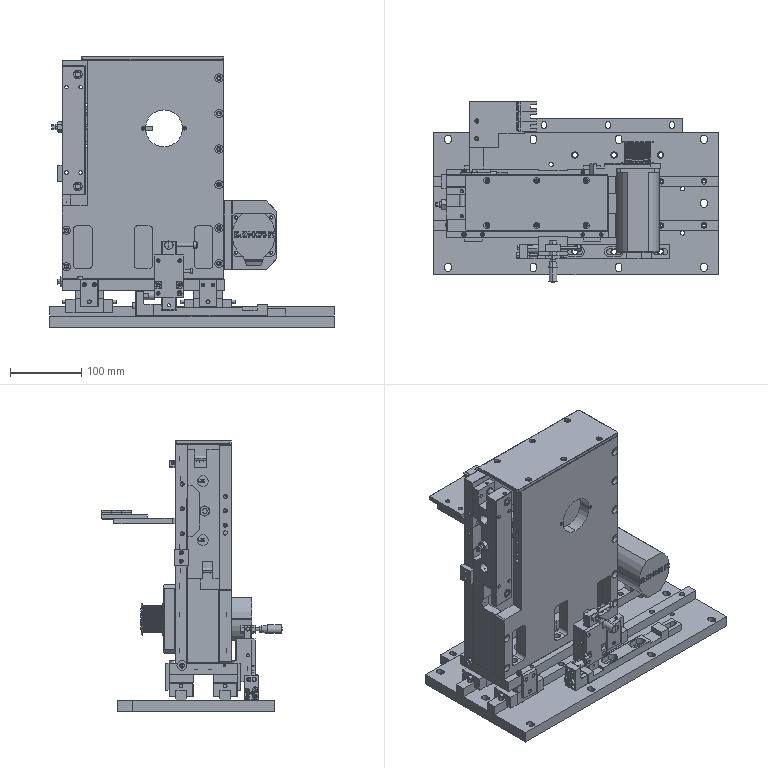Part | NX | 74 solids | 4442 faces | volume 5162525 mm3 | plane 2231 | cylinder 1481 | cone 676 | spline 44 | sphere 6 | torus 4 | commonest cylinder face diameters 5 x427 3.3 x150 4.5 x64 6.6 x54 0.5 x52 4.2 x52